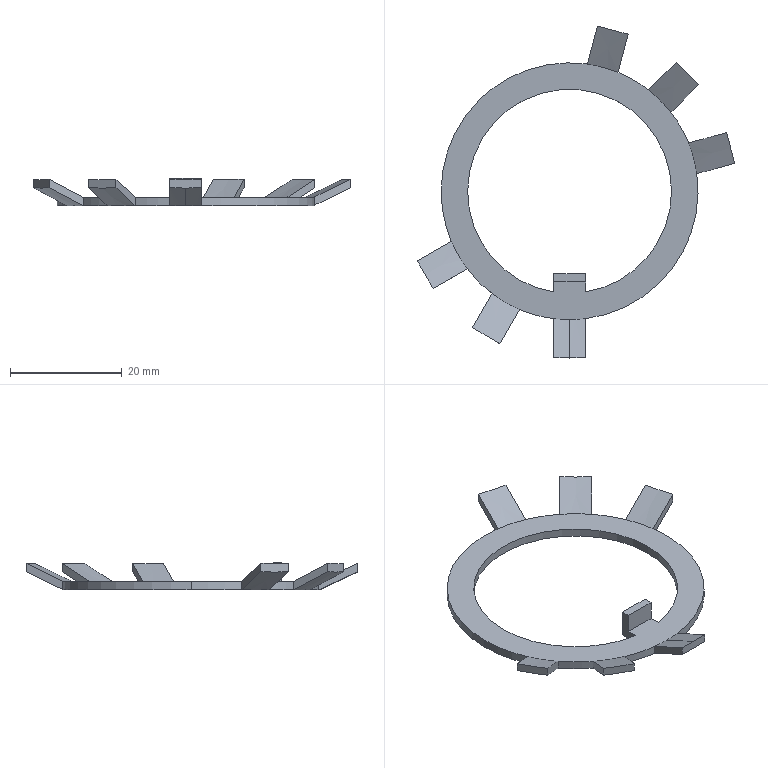Part | SolidWorks | features Boss 1, Cut 1, Revolution 1 | 1 solid | 49 faces | box 56.873 x 59.449 x 5 mm | volume 1338 mm3 | plane 25 | cone 14 | cylinder 10 | commonest cylinder face diameters 46 x7 36.5 x3
STEP:
#1=CARTESIAN_POINT('',(0.,-23.,0.));
#2=VERTEX_POINT('',#1);
#3=CARTESIAN_POINT('',(-2.85,-22.823,0.));
#4=VERTEX_POINT('',#3);
#5=CARTESIAN_POINT('',(0.,0.,0.));
#6=DIRECTION('',(0.,0.,-1.));
#7=DIRECTION('',(0.,1.,0.));
#8=AXIS2_PLACEMENT_3D('',#5,#6,#7);
#9=CIRCLE('',#8,23.);
#10=EDGE_CURVE('',#2,#4,#9,.T.);
#11=ORIENTED_EDGE('',*,*,#10,.F.);
#12=CARTESIAN_POINT('',(0.,-29.864,3.201));
#13=VERTEX_POINT('',#12);
#14=CARTESIAN_POINT('',(0.,-23.,0.));
#15=DIRECTION('',(0.,-0.9063,0.4226));
#16=VECTOR('',#15,1000.);
#17=LINE('',#14,#16);
#18=EDGE_CURVE('',#2,#13,#17,.T.);
#19=ORIENTED_EDGE('',*,*,#18,.T.);
#20=CARTESIAN_POINT('',(-2.85,-29.864,3.264));
#21=VERTEX_POINT('',#20);
#22=CARTESIAN_POINT('',(0.,-29.864,3.201));
#23=CARTESIAN_POINT('',(-0.9489,-29.864,3.201));
#24=CARTESIAN_POINT('',(-1.9,-29.864,3.222));
#25=CARTESIAN_POINT('',(-2.85,-29.864,3.264));
#26=B_SPLINE_CURVE_WITH_KNOTS('',3,(#22,#23,#24,#25),.UNSPECIFIED.,.F.,.F.,(4,4),(0.01086,0.0137),.UNSPECIFIED.);
#27=EDGE_CURVE('',#13,#21,#26,.T.);
#28=ORIENTED_EDGE('',*,*,#27,.T.);
#29=CARTESIAN_POINT('',(-2.85,-29.864,3.264));
#30=CARTESIAN_POINT('',(-2.85,-27.518,2.175));
#31=CARTESIAN_POINT('',(-2.85,-25.171,1.086));
#32=CARTESIAN_POINT('',(-2.85,-22.823,0.));
#33=B_SPLINE_CURVE_WITH_KNOTS('',3,(#29,#30,#31,#32),.UNSPECIFIED.,.F.,.F.,(4,4),(0.01434,0.02211),.UNSPECIFIED.);
#34=EDGE_CURVE('',#21,#4,#33,.T.);
#35=ORIENTED_EDGE('',*,*,#34,.T.);
#36=EDGE_LOOP('',(#11,#19,#28,#35));
#37=FACE_OUTER_BOUND('',#36,.T.);
#38=CARTESIAN_POINT('',(0.,0.,0.));
#39=DIRECTION('',(0.,0.,1.));
#40=DIRECTION('',(0.,-1.,0.));
#41=AXIS2_PLACEMENT_3D('',#38,#39,#40);
#42=CONICAL_SURFACE('',#41,23.,1.134);
#43=ADVANCED_FACE('',(#37),#42,.T.);
#44=CARTESIAN_POINT('',(-21.19,-8.943,1.5));
#45=VERTEX_POINT('',#44);
#46=CARTESIAN_POINT('',(-23.,0.,1.5));
#47=VERTEX_POINT('',#46);
#48=CARTESIAN_POINT('',(0.,0.,1.5));
#49=DIRECTION('',(0.,0.,-1.));
#50=DIRECTION('',(0.,1.,0.));
#51=AXIS2_PLACEMENT_3D('',#48,#49,#50);
#52=CIRCLE('',#51,23.);
#53=EDGE_CURVE('',#45,#47,#52,.T.);
#54=ORIENTED_EDGE('',*,*,#53,.T.);
#55=CARTESIAN_POINT('',(-23.,0.,0.));
#56=VERTEX_POINT('',#55);
#57=CARTESIAN_POINT('',(-23.,0.,4.765));
#58=DIRECTION('',(0.,0.,-1.));
#59=VECTOR('',#58,1000.);
#60=LINE('',#57,#59);
#61=EDGE_CURVE('',#47,#56,#60,.T.);
#62=ORIENTED_EDGE('',*,*,#61,.T.);
#63=CARTESIAN_POINT('',(-21.19,-8.943,0.));
#64=VERTEX_POINT('',#63);
#65=CARTESIAN_POINT('',(0.,0.,0.));
#66=DIRECTION('',(0.,0.,1.));
#67=DIRECTION('',(1.,0.,0.));
#68=AXIS2_PLACEMENT_3D('',#65,#66,#67);
#69=CIRCLE('',#68,23.);
#70=EDGE_CURVE('',#56,#64,#69,.T.);
#71=ORIENTED_EDGE('',*,*,#70,.T.);
#72=CARTESIAN_POINT('',(-21.19,-8.943,4.765));
#73=DIRECTION('',(0.,0.,-1.));
#74=VECTOR('',#73,1000.);
#75=LINE('',#72,#74);
#76=EDGE_CURVE('',#45,#64,#75,.T.);
#77=ORIENTED_EDGE('',*,*,#76,.F.);
#78=EDGE_LOOP('',(#54,#62,#71,#77));
#79=FACE_OUTER_BOUND('',#78,.T.);
#80=CARTESIAN_POINT('',(0.,0.,4.765));
#81=DIRECTION('',(0.,0.,-1.));
#82=DIRECTION('',(-1.,0.,0.));
#83=AXIS2_PLACEMENT_3D('',#80,#81,#82);
#84=CYLINDRICAL_SURFACE('',#83,23.);
#85=ADVANCED_FACE('',(#79),#84,.T.);
#86=CARTESIAN_POINT('',(2.85,-18.026,1.5));
#87=VERTEX_POINT('',#86);
#88=CARTESIAN_POINT('',(18.25,0.,1.5));
#89=VERTEX_POINT('',#88);
#90=CARTESIAN_POINT('',(0.,0.,1.5));
#91=DIRECTION('',(0.,0.,1.));
#92=DIRECTION('',(0.,-1.,0.));
#93=AXIS2_PLACEMENT_3D('',#90,#91,#92);
#94=CIRCLE('',#93,18.25);
#95=EDGE_CURVE('',#87,#89,#94,.T.);
#96=ORIENTED_EDGE('',*,*,#95,.T.);
#97=CARTESIAN_POINT('',(18.25,0.,0.));
#98=VERTEX_POINT('',#97);
#99=CARTESIAN_POINT('',(18.25,0.,4.765));
#100=DIRECTION('',(0.,0.,-1.));
#101=VECTOR('',#100,1000.);
#102=LINE('',#99,#101);
#103=EDGE_CURVE('',#89,#98,#102,.T.);
#104=ORIENTED_EDGE('',*,*,#103,.T.);
#105=CARTESIAN_POINT('',(2.85,-18.026,0.));
#106=VERTEX_POINT('',#105);
#107=CARTESIAN_POINT('',(0.,0.,0.));
#108=DIRECTION('',(0.,0.,1.));
#109=DIRECTION('',(1.,0.,0.));
#110=AXIS2_PLACEMENT_3D('',#107,#108,#109);
#111=CIRCLE('',#110,18.25);
#112=EDGE_CURVE('',#106,#98,#111,.T.);
#113=ORIENTED_EDGE('',*,*,#112,.F.);
#114=CARTESIAN_POINT('',(2.85,-18.026,4.765));
#115=DIRECTION('',(0.,0.,-1.));
#116=VECTOR('',#115,1000.);
#117=LINE('',#114,#116);
#118=EDGE_CURVE('',#87,#106,#117,.T.);
#119=ORIENTED_EDGE('',*,*,#118,.F.);
#120=EDGE_LOOP('',(#96,#104,#113,#119));
#121=FACE_OUTER_BOUND('',#120,.T.);
#122=CARTESIAN_POINT('',(0.,0.,4.765));
#123=DIRECTION('',(0.,0.,-1.));
#124=DIRECTION('',(-1.,0.,0.));
#125=AXIS2_PLACEMENT_3D('',#122,#123,#124);
#126=CYLINDRICAL_SURFACE('',#125,18.25);
#127=ADVANCED_FACE('',(#121),#126,.F.);
#128=ORIENTED_EDGE('',*,*,#103,.F.);
#129=CARTESIAN_POINT('',(-18.25,0.,1.5));
#130=VERTEX_POINT('',#129);
#131=CARTESIAN_POINT('',(0.,0.,1.5));
#132=DIRECTION('',(0.,0.,1.));
#133=DIRECTION('',(0.,-1.,0.));
#134=AXIS2_PLACEMENT_3D('',#131,#132,#133);
#135=CIRCLE('',#134,18.25);
#136=EDGE_CURVE('',#89,#130,#135,.T.);
#137=ORIENTED_EDGE('',*,*,#136,.T.);
#138=CARTESIAN_POINT('',(-18.25,0.,0.));
#139=VERTEX_POINT('',#138);
#140=CARTESIAN_POINT('',(-18.25,0.,4.765));
#141=DIRECTION('',(0.,0.,-1.));
#142=VECTOR('',#141,1000.);
#143=LINE('',#140,#142);
#144=EDGE_CURVE('',#130,#139,#143,.T.);
#145=ORIENTED_EDGE('',*,*,#144,.T.);
#146=CARTESIAN_POINT('',(0.,0.,0.));
#147=DIRECTION('',(0.,0.,1.));
#148=DIRECTION('',(1.,0.,0.));
#149=AXIS2_PLACEMENT_3D('',#146,#147,#148);
#150=CIRCLE('',#149,18.25);
#151=EDGE_CURVE('',#98,#139,#150,.T.);
#152=ORIENTED_EDGE('',*,*,#151,.F.);
#153=EDGE_LOOP('',(#128,#137,#145,#152));
#154=FACE_OUTER_BOUND('',#153,.T.);
#155=CARTESIAN_POINT('',(0.,0.,4.765));
#156=DIRECTION('',(0.,0.,-1.));
#157=DIRECTION('',(-1.,0.,0.));
#158=AXIS2_PLACEMENT_3D('',#155,#156,#157);
#159=CYLINDRICAL_SURFACE('',#158,18.25);
#160=ADVANCED_FACE('',(#154),#159,.F.);
#161=CARTESIAN_POINT('',(2.85,-22.823,1.5));
#162=VERTEX_POINT('',#161);
#163=CARTESIAN_POINT('',(0.,-23.,1.5));
#164=VERTEX_POINT('',#163);
#165=CARTESIAN_POINT('',(0.,0.,1.5));
#166=DIRECTION('',(0.,0.,-1.));
#167=DIRECTION('',(0.,1.,0.));
#168=AXIS2_PLACEMENT_3D('',#165,#166,#167);
#169=CIRCLE('',#168,23.);
#170=EDGE_CURVE('',#162,#164,#169,.T.);
#171=ORIENTED_EDGE('',*,*,#170,.T.);
#172=CARTESIAN_POINT('',(0.,-29.864,4.701));
#173=VERTEX_POINT('',#172);
#174=CARTESIAN_POINT('',(0.,-30.,4.764));
#175=DIRECTION('',(0.,-0.9063,0.4226));
#176=VECTOR('',#175,1000.);
#177=LINE('',#174,#176);
#178=EDGE_CURVE('',#164,#173,#177,.T.);
#179=ORIENTED_EDGE('',*,*,#178,.T.);
#180=CARTESIAN_POINT('',(2.85,-29.864,4.764));
#181=VERTEX_POINT('',#180);
#182=CARTESIAN_POINT('',(0.,-29.864,4.701));
#183=CARTESIAN_POINT('',(0.9514,-29.864,4.701));
#184=CARTESIAN_POINT('',(1.901,-29.864,4.722));
#185=CARTESIAN_POINT('',(2.85,-29.864,4.764));
#186=B_SPLINE_CURVE_WITH_KNOTS('',3,(#182,#183,#184,#185),.UNSPECIFIED.,.F.,.F.,(4,4),(0.01506,0.01791),.UNSPECIFIED.);
#187=EDGE_CURVE('',#173,#181,#186,.T.);
#188=ORIENTED_EDGE('',*,*,#187,.T.);
#189=CARTESIAN_POINT('',(2.85,-29.864,4.764));
#190=CARTESIAN_POINT('',(2.85,-27.518,3.675));
#191=CARTESIAN_POINT('',(2.85,-25.171,2.586));
#192=CARTESIAN_POINT('',(2.85,-22.823,1.5));
#193=B_SPLINE_CURVE_WITH_KNOTS('',3,(#189,#190,#191,#192),.UNSPECIFIED.,.F.,.F.,(4,4),(0.01434,0.02211),.UNSPECIFIED.);
#194=EDGE_CURVE('',#181,#162,#193,.T.);
#195=ORIENTED_EDGE('',*,*,#194,.T.);
#196=EDGE_LOOP('',(#171,#179,#188,#195));
#197=FACE_OUTER_BOUND('',#196,.T.);
#198=CARTESIAN_POINT('',(0.,0.,4.764));
#199=DIRECTION('',(0.,0.,1.));
#200=DIRECTION('',(0.,-1.,0.));
#201=AXIS2_PLACEMENT_3D('',#198,#199,#200);
#202=CONICAL_SURFACE('',#201,30.,1.134);
#203=ADVANCED_FACE('',(#197),#202,.F.);
#204=CARTESIAN_POINT('',(3.154,22.783,1.5));
#205=VERTEX_POINT('',#204);
#206=CARTESIAN_POINT('',(8.66,21.307,1.5));
#207=VERTEX_POINT('',#206);
#208=CARTESIAN_POINT('',(0.,0.,1.5));
#209=DIRECTION('',(0.,0.,-1.));
#210=DIRECTION('',(0.,1.,0.));
#211=AXIS2_PLACEMENT_3D('',#208,#209,#210);
#212=CIRCLE('',#211,23.);
#213=EDGE_CURVE('',#205,#207,#212,.T.);
#214=ORIENTED_EDGE('',*,*,#213,.F.);
#215=CARTESIAN_POINT('',(0.,0.,1.5));
#216=DIRECTION('',(0.,0.,-1.));
#217=DIRECTION('',(0.,1.,0.));
#218=AXIS2_PLACEMENT_3D('',#215,#216,#217);
#219=CIRCLE('',#218,23.);
#220=EDGE_CURVE('',#47,#205,#219,.T.);
#221=ORIENTED_EDGE('',*,*,#220,.F.);
#222=ORIENTED_EDGE('',*,*,#53,.F.);
#223=CARTESIAN_POINT('',(-18.34,-13.88,1.5));
#224=VERTEX_POINT('',#223);
#225=CARTESIAN_POINT('',(0.,0.,1.5));
#226=DIRECTION('',(0.,0.,-1.));
#227=DIRECTION('',(0.,1.,0.));
#228=AXIS2_PLACEMENT_3D('',#225,#226,#227);
#229=CIRCLE('',#228,23.);
#230=EDGE_CURVE('',#224,#45,#229,.T.);
#231=ORIENTED_EDGE('',*,*,#230,.F.);
#232=CARTESIAN_POINT('',(-13.88,-18.34,1.5));
#233=VERTEX_POINT('',#232);
#234=CARTESIAN_POINT('',(0.,0.,1.5));
#235=DIRECTION('',(0.,0.,-1.));
#236=DIRECTION('',(0.,1.,0.));
#237=AXIS2_PLACEMENT_3D('',#234,#235,#236);
#238=CIRCLE('',#237,23.);
#239=EDGE_CURVE('',#233,#224,#238,.T.);
#240=ORIENTED_EDGE('',*,*,#239,.F.);
#241=CARTESIAN_POINT('',(-8.943,-21.19,1.5));
#242=VERTEX_POINT('',#241);
#243=CARTESIAN_POINT('',(0.,0.,1.5));
#244=DIRECTION('',(0.,0.,-1.));
#245=DIRECTION('',(0.,1.,0.));
#246=AXIS2_PLACEMENT_3D('',#243,#244,#245);
#247=CIRCLE('',#246,23.);
#248=EDGE_CURVE('',#242,#233,#247,.T.);
#249=ORIENTED_EDGE('',*,*,#248,.F.);
#250=CARTESIAN_POINT('',(-2.85,-22.823,1.5));
#251=VERTEX_POINT('',#250);
#252=CARTESIAN_POINT('',(0.,0.,1.5));
#253=DIRECTION('',(0.,0.,-1.));
#254=DIRECTION('',(0.,1.,0.));
#255=AXIS2_PLACEMENT_3D('',#252,#253,#254);
#256=CIRCLE('',#255,23.);
#257=EDGE_CURVE('',#251,#242,#256,.T.);
#258=ORIENTED_EDGE('',*,*,#257,.F.);
#259=CARTESIAN_POINT('',(0.,0.,1.5));
#260=DIRECTION('',(0.,0.,-1.));
#261=DIRECTION('',(0.,1.,0.));
#262=AXIS2_PLACEMENT_3D('',#259,#260,#261);
#263=CIRCLE('',#262,23.);
#264=EDGE_CURVE('',#164,#251,#263,.T.);
#265=ORIENTED_EDGE('',*,*,#264,.F.);
#266=ORIENTED_EDGE('',*,*,#170,.F.);
#267=CARTESIAN_POINT('',(22.783,3.154,1.5));
#268=VERTEX_POINT('',#267);
#269=CARTESIAN_POINT('',(0.,0.,1.5));
#270=DIRECTION('',(0.,0.,-1.));
#271=DIRECTION('',(0.,1.,0.));
#272=AXIS2_PLACEMENT_3D('',#269,#270,#271);
#273=CIRCLE('',#272,23.);
#274=EDGE_CURVE('',#268,#162,#273,.T.);
#275=ORIENTED_EDGE('',*,*,#274,.F.);
#276=CARTESIAN_POINT('',(21.307,8.66,1.5));
#277=VERTEX_POINT('',#276);
#278=CARTESIAN_POINT('',(0.,0.,1.5));
#279=DIRECTION('',(0.,0.,-1.));
#280=DIRECTION('',(0.,1.,0.));
#281=AXIS2_PLACEMENT_3D('',#278,#279,#280);
#282=CIRCLE('',#281,23.);
#283=EDGE_CURVE('',#277,#268,#282,.T.);
#284=ORIENTED_EDGE('',*,*,#283,.F.);
#285=CARTESIAN_POINT('',(18.153,14.123,1.5));
#286=VERTEX_POINT('',#285);
#287=CARTESIAN_POINT('',(0.,0.,1.5));
#288=DIRECTION('',(0.,0.,-1.));
#289=DIRECTION('',(0.,1.,0.));
#290=AXIS2_PLACEMENT_3D('',#287,#288,#289);
#291=CIRCLE('',#290,23.);
#292=EDGE_CURVE('',#286,#277,#291,.T.);
#293=ORIENTED_EDGE('',*,*,#292,.F.);
#294=CARTESIAN_POINT('',(14.123,18.153,1.5));
#295=VERTEX_POINT('',#294);
#296=CARTESIAN_POINT('',(0.,0.,1.5));
#297=DIRECTION('',(0.,0.,-1.));
#298=DIRECTION('',(0.,1.,0.));
#299=AXIS2_PLACEMENT_3D('',#296,#297,#298);
#300=CIRCLE('',#299,23.);
#301=EDGE_CURVE('',#295,#286,#300,.T.);
#302=ORIENTED_EDGE('',*,*,#301,.F.);
#303=CARTESIAN_POINT('',(0.,0.,1.5));
#304=DIRECTION('',(0.,0.,-1.));
#305=DIRECTION('',(0.,1.,0.));
#306=AXIS2_PLACEMENT_3D('',#303,#304,#305);
#307=CIRCLE('',#306,23.);
#308=EDGE_CURVE('',#207,#295,#307,.T.);
#309=ORIENTED_EDGE('',*,*,#308,.F.);
#310=EDGE_LOOP('',(#214,#221,#222,#231,#240,#249,#258,#265,#266,#275,#284,#293,#302,#309));
#311=FACE_OUTER_BOUND('',#310,.T.);
#312=CARTESIAN_POINT('',(2.85,-16.25,1.5));
#313=VERTEX_POINT('',#312);
#314=CARTESIAN_POINT('',(2.85,-18.026,1.5));
#315=DIRECTION('',(0.,-1.,0.));
#316=VECTOR('',#315,1000.);
#317=LINE('',#314,#316);
#318=EDGE_CURVE('',#313,#87,#317,.T.);
#319=ORIENTED_EDGE('',*,*,#318,.F.);
#320=CARTESIAN_POINT('',(-2.85,-16.25,1.5));
#321=VERTEX_POINT('',#320);
#322=CARTESIAN_POINT('',(0.,-16.25,1.5));
#323=DIRECTION('',(-1.,0.,0.));
#324=VECTOR('',#323,1000.);
#325=LINE('',#322,#324);
#326=EDGE_CURVE('',#313,#321,#325,.T.);
#327=ORIENTED_EDGE('',*,*,#326,.T.);
#328=CARTESIAN_POINT('',(-2.85,-18.026,1.5));
#329=VERTEX_POINT('',#328);
#330=CARTESIAN_POINT('',(-2.85,-18.026,1.5));
#331=DIRECTION('',(0.,1.,0.));
#332=VECTOR('',#331,1000.);
#333=LINE('',#330,#332);
#334=EDGE_CURVE('',#329,#321,#333,.T.);
#335=ORIENTED_EDGE('',*,*,#334,.F.);
#336=CARTESIAN_POINT('',(0.,0.,1.5));
#337=DIRECTION('',(0.,0.,1.));
#338=DIRECTION('',(0.,-1.,0.));
#339=AXIS2_PLACEMENT_3D('',#336,#337,#338);
#340=CIRCLE('',#339,18.25);
#341=EDGE_CURVE('',#130,#329,#340,.T.);
#342=ORIENTED_EDGE('',*,*,#341,.F.);
#343=ORIENTED_EDGE('',*,*,#136,.F.);
#344=ORIENTED_EDGE('',*,*,#95,.F.);
#345=EDGE_LOOP('',(#319,#327,#335,#342,#343,#344));
#346=FACE_BOUND('',#345,.T.);
#347=CARTESIAN_POINT('',(0.,23.,1.5));
#348=DIRECTION('',(0.,0.,1.));
#349=DIRECTION('',(0.,-1.,0.));
#350=AXIS2_PLACEMENT_3D('',#347,#348,#349);
#351=PLANE('',#350);
#352=ADVANCED_FACE('',(#311,#346),#351,.T.);
#353=ORIENTED_EDGE('',*,*,#178,.F.);
#354=ORIENTED_EDGE('',*,*,#264,.T.);
#355=CARTESIAN_POINT('',(-2.85,-29.864,4.764));
#356=VERTEX_POINT('',#355);
#357=CARTESIAN_POINT('',(-2.85,-22.823,1.5));
#358=CARTESIAN_POINT('',(-2.85,-25.171,2.586));
#359=CARTESIAN_POINT('',(-2.85,-27.518,3.675));
#360=CARTESIAN_POINT('',(-2.85,-29.864,4.764));
#361=B_SPLINE_CURVE_WITH_KNOTS('',3,(#357,#358,#359,#360),.UNSPECIFIED.,.F.,.F.,(4,4),(0.008867,0.01663),.UNSPECIFIED.);
#362=EDGE_CURVE('',#251,#356,#361,.T.);
#363=ORIENTED_EDGE('',*,*,#362,.T.);
#364=CARTESIAN_POINT('',(-2.85,-29.864,4.764));
#365=CARTESIAN_POINT('',(-1.9,-29.864,4.722));
#366=CARTESIAN_POINT('',(-0.9489,-29.864,4.701));
#367=CARTESIAN_POINT('',(0.,-29.864,4.701));
#368=B_SPLINE_CURVE_WITH_KNOTS('',3,(#364,#365,#366,#367),.UNSPECIFIED.,.F.,.F.,(4,4),(0.01222,0.01506),.UNSPECIFIED.);
#369=EDGE_CURVE('',#356,#173,#368,.T.);
#370=ORIENTED_EDGE('',*,*,#369,.T.);
#371=EDGE_LOOP('',(#353,#354,#363,#370));
#372=FACE_OUTER_BOUND('',#371,.T.);
#373=CARTESIAN_POINT('',(0.,0.,4.764));
#374=DIRECTION('',(0.,0.,1.));
#375=DIRECTION('',(0.,-1.,0.));
#376=AXIS2_PLACEMENT_3D('',#373,#374,#375);
#377=CONICAL_SURFACE('',#376,30.,1.134);
#378=ADVANCED_FACE('',(#372),#377,.F.);
#379=CARTESIAN_POINT('',(-17.4,-24.438,4.764));
#380=VERTEX_POINT('',#379);
#381=CARTESIAN_POINT('',(-13.88,-18.34,1.5));
#382=CARTESIAN_POINT('',(-15.054,-20.373,2.586));
#383=CARTESIAN_POINT('',(-16.227,-22.406,3.675));
#384=CARTESIAN_POINT('',(-17.4,-24.438,4.764));
#385=B_SPLINE_CURVE_WITH_KNOTS('',3,(#381,#382,#383,#384),.UNSPECIFIED.,.F.,.F.,(4,4),(0.000000255,0.007762),.UNSPECIFIED.);
#386=EDGE_CURVE('',#233,#380,#385,.T.);
#387=ORIENTED_EDGE('',*,*,#386,.T.);
#388=CARTESIAN_POINT('',(-12.464,-27.288,4.764));
#389=VERTEX_POINT('',#388);
#390=CARTESIAN_POINT('',(-17.4,-24.438,4.764));
#391=CARTESIAN_POINT('',(-15.755,-25.388,4.68));
#392=CARTESIAN_POINT('',(-14.109,-26.338,4.68));
#393=CARTESIAN_POINT('',(-12.464,-27.288,4.764));
#394=B_SPLINE_CURVE_WITH_KNOTS('',3,(#390,#391,#392,#393),.UNSPECIFIED.,.F.,.F.,(4,4),(0.000000231,0.0057),.UNSPECIFIED.);
#395=EDGE_CURVE('',#380,#389,#394,.T.);
#396=ORIENTED_EDGE('',*,*,#395,.T.);
#397=CARTESIAN_POINT('',(-12.464,-27.288,4.764));
#398=CARTESIAN_POINT('',(-11.291,-25.256,3.675));
#399=CARTESIAN_POINT('',(-10.117,-23.223,2.586));
#400=CARTESIAN_POINT('',(-8.943,-21.19,1.5));
#401=B_SPLINE_CURVE_WITH_KNOTS('',3,(#397,#398,#399,#400),.UNSPECIFIED.,.F.,.F.,(4,4),(0.000000255,0.007762),.UNSPECIFIED.);
#402=EDGE_CURVE('',#389,#242,#401,.T.);
#403=ORIENTED_EDGE('',*,*,#402,.T.);
#404=ORIENTED_EDGE('',*,*,#248,.T.);
#405=EDGE_LOOP('',(#387,#396,#403,#404));
#406=FACE_OUTER_BOUND('',#405,.T.);
#407=CARTESIAN_POINT('',(0.,0.,4.764));
#408=DIRECTION('',(0.,0.,1.));
#409=DIRECTION('',(0.,-1.,0.));
#410=AXIS2_PLACEMENT_3D('',#407,#408,#409);
#411=CONICAL_SURFACE('',#410,30.,1.134);
#412=ADVANCED_FACE('',(#406),#411,.F.);
#413=CARTESIAN_POINT('',(-27.288,-12.464,4.764));
#414=VERTEX_POINT('',#413);
#415=CARTESIAN_POINT('',(-21.19,-8.943,1.5));
#416=CARTESIAN_POINT('',(-23.223,-10.117,2.586));
#417=CARTESIAN_POINT('',(-25.256,-11.291,3.675));
#418=CARTESIAN_POINT('',(-27.288,-12.464,4.764));
#419=B_SPLINE_CURVE_WITH_KNOTS('',3,(#415,#416,#417,#418),.UNSPECIFIED.,.F.,.F.,(4,4),(0.000000255,0.007762),.UNSPECIFIED.);
#420=EDGE_CURVE('',#45,#414,#419,.T.);
#421=ORIENTED_EDGE('',*,*,#420,.T.);
#422=CARTESIAN_POINT('',(-24.438,-17.4,4.764));
#423=VERTEX_POINT('',#422);
#424=CARTESIAN_POINT('',(-27.288,-12.464,4.764));
#425=CARTESIAN_POINT('',(-26.338,-14.109,4.68));
#426=CARTESIAN_POINT('',(-25.388,-15.755,4.68));
#427=CARTESIAN_POINT('',(-24.438,-17.4,4.764));
#428=B_SPLINE_CURVE_WITH_KNOTS('',3,(#424,#425,#426,#427),.UNSPECIFIED.,.F.,.F.,(4,4),(0.000000231,0.0057),.UNSPECIFIED.);
#429=EDGE_CURVE('',#414,#423,#428,.T.);
#430=ORIENTED_EDGE('',*,*,#429,.T.);
#431=CARTESIAN_POINT('',(-24.438,-17.4,4.764));
#432=CARTESIAN_POINT('',(-22.406,-16.227,3.675));
#433=CARTESIAN_POINT('',(-20.373,-15.054,2.586));
#434=CARTESIAN_POINT('',(-18.34,-13.88,1.5));
#435=B_SPLINE_CURVE_WITH_KNOTS('',3,(#431,#432,#433,#434),.UNSPECIFIED.,.F.,.F.,(4,4),(0.000000255,0.007762),.UNSPECIFIED.);
#436=EDGE_CURVE('',#423,#224,#435,.T.);
#437=ORIENTED_EDGE('',*,*,#436,.T.);
#438=ORIENTED_EDGE('',*,*,#230,.T.);
#439=EDGE_LOOP('',(#421,#430,#437,#438));
#440=FACE_OUTER_BOUND('',#439,.T.);
#441=CARTESIAN_POINT('',(0.,0.,4.764));
#442=DIRECTION('',(0.,0.,1.));
#443=DIRECTION('',(0.,-1.,0.));
#444=AXIS2_PLACEMENT_3D('',#441,#442,#443);
#445=CONICAL_SURFACE('',#444,30.,1.134);
#446=ADVANCED_FACE('',(#440),#445,.F.);
#447=CARTESIAN_POINT('',(10.482,28.109,4.764));
#448=VERTEX_POINT('',#447);
#449=CARTESIAN_POINT('',(8.66,21.307,1.5));
#450=CARTESIAN_POINT('',(9.268,23.575,2.586));
#451=CARTESIAN_POINT('',(9.875,25.842,3.675));
#452=CARTESIAN_POINT('',(10.482,28.109,4.764));
#453=B_SPLINE_CURVE_WITH_KNOTS('',3,(#449,#450,#451,#452),.UNSPECIFIED.,.F.,.F.,(4,4),(0.000000228,0.007762),.UNSPECIFIED.);
#454=EDGE_CURVE('',#207,#448,#453,.T.);
#455=ORIENTED_EDGE('',*,*,#454,.T.);
#456=CARTESIAN_POINT('',(4.977,29.584,4.764));
#457=VERTEX_POINT('',#456);
#458=CARTESIAN_POINT('',(10.482,28.109,4.764));
#459=CARTESIAN_POINT('',(8.647,28.601,4.68));
#460=CARTESIAN_POINT('',(6.812,29.093,4.68));
#461=CARTESIAN_POINT('',(4.977,29.584,4.764));
#462=B_SPLINE_CURVE_WITH_KNOTS('',3,(#458,#459,#460,#461),.UNSPECIFIED.,.F.,.F.,(4,4),(0.000000207,0.0057),.UNSPECIFIED.);
#463=EDGE_CURVE('',#448,#457,#462,.T.);
#464=ORIENTED_EDGE('',*,*,#463,.T.);
#465=CARTESIAN_POINT('',(4.977,29.584,4.764));
#466=CARTESIAN_POINT('',(4.369,27.318,3.675));
#467=CARTESIAN_POINT('',(3.762,25.051,2.586));
#468=CARTESIAN_POINT('',(3.154,22.783,1.5));
#469=B_SPLINE_CURVE_WITH_KNOTS('',3,(#465,#466,#467,#468),.UNSPECIFIED.,.F.,.F.,(4,4),(0.000000228,0.007762),.UNSPECIFIED.);
#470=EDGE_CURVE('',#457,#205,#469,.T.);
#471=ORIENTED_EDGE('',*,*,#470,.T.);
#472=ORIENTED_EDGE('',*,*,#213,.T.);
#473=EDGE_LOOP('',(#455,#464,#471,#472));
#474=FACE_OUTER_BOUND('',#473,.T.);
#475=CARTESIAN_POINT('',(0.,0.,4.764));
#476=DIRECTION('',(0.,0.,1.));
#477=DIRECTION('',(0.,-1.,0.));
#478=AXIS2_PLACEMENT_3D('',#475,#476,#477);
#479=CONICAL_SURFACE('',#478,30.,1.134);
#480=ADVANCED_FACE('',(#474),#479,.F.);
#481=CARTESIAN_POINT('',(23.133,19.102,4.764));
#482=VERTEX_POINT('',#481);
#483=CARTESIAN_POINT('',(18.153,14.123,1.5));
#484=CARTESIAN_POINT('',(19.814,15.783,2.586));
#485=CARTESIAN_POINT('',(21.473,17.443,3.675));
#486=CARTESIAN_POINT('',(23.133,19.102,4.764));
#487=B_SPLINE_CURVE_WITH_KNOTS('',3,(#483,#484,#485,#486),.UNSPECIFIED.,.F.,.F.,(4,4),(0.000000312,0.007762),.UNSPECIFIED.);
#488=EDGE_CURVE('',#286,#482,#487,.T.);
#489=ORIENTED_EDGE('',*,*,#488,.T.);
#490=CARTESIAN_POINT('',(19.102,23.133,4.764));
#491=VERTEX_POINT('',#490);
#492=CARTESIAN_POINT('',(23.133,19.102,4.764));
#493=CARTESIAN_POINT('',(21.789,20.446,4.68));
#494=CARTESIAN_POINT('',(20.446,21.789,4.68));
#495=CARTESIAN_POINT('',(19.102,23.133,4.764));
#496=B_SPLINE_CURVE_WITH_KNOTS('',3,(#492,#493,#494,#495),.UNSPECIFIED.,.F.,.F.,(4,4),(0.000000283,0.0057),.UNSPECIFIED.);
#497=EDGE_CURVE('',#482,#491,#496,.T.);
#498=ORIENTED_EDGE('',*,*,#497,.T.);
#499=CARTESIAN_POINT('',(19.102,23.133,4.764));
#500=CARTESIAN_POINT('',(17.443,21.473,3.675));
#501=CARTESIAN_POINT('',(15.783,19.814,2.586));
#502=CARTESIAN_POINT('',(14.123,18.153,1.5));
#503=B_SPLINE_CURVE_WITH_KNOTS('',3,(#499,#500,#501,#502),.UNSPECIFIED.,.F.,.F.,(4,4),(0.000000312,0.007762),.UNSPECIFIED.);
#504=EDGE_CURVE('',#491,#295,#503,.T.);
#505=ORIENTED_EDGE('',*,*,#504,.T.);
#506=ORIENTED_EDGE('',*,*,#301,.T.);
#507=EDGE_LOOP('',(#489,#498,#505,#506));
#508=FACE_OUTER_BOUND('',#507,.T.);
#509=CARTESIAN_POINT('',(0.,0.,4.764));
#510=DIRECTION('',(0.,0.,1.));
#511=DIRECTION('',(0.,-1.,0.));
#512=AXIS2_PLACEMENT_3D('',#509,#510,#511);
#513=CONICAL_SURFACE('',#512,30.,1.134);
#514=ADVANCED_FACE('',(#508),#513,.F.);
#515=CARTESIAN_POINT('',(29.584,4.977,4.764));
#516=VERTEX_POINT('',#515);
#517=CARTESIAN_POINT('',(22.783,3.154,1.5));
#518=CARTESIAN_POINT('',(25.051,3.762,2.586));
#519=CARTESIAN_POINT('',(27.318,4.369,3.675));
#520=CARTESIAN_POINT('',(29.584,4.977,4.764));
#521=B_SPLINE_CURVE_WITH_KNOTS('',3,(#517,#518,#519,#520),.UNSPECIFIED.,.F.,.F.,(4,4),(0.000000228,0.007762),.UNSPECIFIED.);
#522=EDGE_CURVE('',#268,#516,#521,.T.);
#523=ORIENTED_EDGE('',*,*,#522,.T.);
#524=CARTESIAN_POINT('',(28.109,10.482,4.764));
#525=VERTEX_POINT('',#524);
#526=CARTESIAN_POINT('',(29.584,4.977,4.764));
#527=CARTESIAN_POINT('',(29.093,6.812,4.68));
#528=CARTESIAN_POINT('',(28.601,8.647,4.68));
#529=CARTESIAN_POINT('',(28.109,10.482,4.764));
#530=B_SPLINE_CURVE_WITH_KNOTS('',3,(#526,#527,#528,#529),.UNSPECIFIED.,.F.,.F.,(4,4),(0.000000207,0.0057),.UNSPECIFIED.);
#531=EDGE_CURVE('',#516,#525,#530,.T.);
#532=ORIENTED_EDGE('',*,*,#531,.T.);
#533=CARTESIAN_POINT('',(28.109,10.482,4.764));
#534=CARTESIAN_POINT('',(25.842,9.875,3.675));
#535=CARTESIAN_POINT('',(23.575,9.268,2.586));
#536=CARTESIAN_POINT('',(21.307,8.66,1.5));
#537=B_SPLINE_CURVE_WITH_KNOTS('',3,(#533,#534,#535,#536),.UNSPECIFIED.,.F.,.F.,(4,4),(0.000000228,0.007762),.UNSPECIFIED.);
#538=EDGE_CURVE('',#525,#277,#537,.T.);
#539=ORIENTED_EDGE('',*,*,#538,.T.);
#540=ORIENTED_EDGE('',*,*,#283,.T.);
#541=EDGE_LOOP('',(#523,#532,#539,#540));
#542=FACE_OUTER_BOUND('',#541,.T.);
#543=CARTESIAN_POINT('',(0.,0.,4.764));
#544=DIRECTION('',(0.,0.,1.));
#545=DIRECTION('',(0.,-1.,0.));
#546=AXIS2_PLACEMENT_3D('',#543,#544,#545);
#547=CONICAL_SURFACE('',#546,30.,1.134);
#548=ADVANCED_FACE('',(#542),#547,.F.);
#549=CARTESIAN_POINT('',(2.85,-14.75,5.));
#550=VERTEX_POINT('',#549);
#551=CARTESIAN_POINT('',(2.85,-14.75,0.));
#552=VERTEX_POINT('',#551);
#553=CARTESIAN_POINT('',(2.85,-14.75,4.765));
#554=DIRECTION('',(0.,0.,-1.));
#555=VECTOR('',#554,1000.);
#556=LINE('',#553,#555);
#557=EDGE_CURVE('',#550,#552,#556,.T.);
#558=ORIENTED_EDGE('',*,*,#557,.F.);
#559=CARTESIAN_POINT('',(2.85,-16.25,5.));
#560=VERTEX_POINT('',#559);
#561=CARTESIAN_POINT('',(2.85,-14.75,5.));
#562=DIRECTION('',(0.,1.,0.));
#563=VECTOR('',#562,1000.);
#564=LINE('',#561,#563);
#565=EDGE_CURVE('',#560,#550,#564,.T.);
#566=ORIENTED_EDGE('',*,*,#565,.F.);
#567=CARTESIAN_POINT('',(2.85,-16.25,5.));
#568=DIRECTION('',(0.,0.,-1.));
#569=VECTOR('',#568,1000.);
#570=LINE('',#567,#569);
#571=EDGE_CURVE('',#560,#313,#570,.T.);
#572=ORIENTED_EDGE('',*,*,#571,.T.);
#573=ORIENTED_EDGE('',*,*,#318,.T.);
#574=ORIENTED_EDGE('',*,*,#118,.T.);
#575=CARTESIAN_POINT('',(2.85,-18.026,0.));
#576=DIRECTION('',(0.,-1.,0.));
#577=VECTOR('',#576,1000.);
#578=LINE('',#575,#577);
#579=EDGE_CURVE('',#552,#106,#578,.T.);
#580=ORIENTED_EDGE('',*,*,#579,.F.);
#581=EDGE_LOOP('',(#558,#566,#572,#573,#574,#580));
#582=FACE_OUTER_BOUND('',#581,.T.);
#583=CARTESIAN_POINT('',(2.85,-18.026,4.765));
#584=DIRECTION('',(1.,0.,0.));
#585=DIRECTION('',(0.,1.,0.));
#586=AXIS2_PLACEMENT_3D('',#583,#584,#585);
#587=PLANE('',#586);
#588=ADVANCED_FACE('',(#582),#587,.T.);
#589=CARTESIAN_POINT('',(-2.85,-14.75,5.));
#590=VERTEX_POINT('',#589);
#591=CARTESIAN_POINT('',(-2.85,-14.75,0.));
#592=VERTEX_POINT('',#591);
#593=CARTESIAN_POINT('',(-2.85,-14.75,4.765));
#594=DIRECTION('',(0.,0.,-1.));
#595=VECTOR('',#594,1000.);
#596=LINE('',#593,#595);
#597=EDGE_CURVE('',#590,#592,#596,.T.);
#598=ORIENTED_EDGE('',*,*,#597,.F.);
#599=CARTESIAN_POINT('',(-2.85,-14.75,5.));
#600=DIRECTION('',(-1.,0.,0.));
#601=VECTOR('',#600,1000.);
#602=LINE('',#599,#601);
#603=EDGE_CURVE('',#550,#590,#602,.T.);
#604=ORIENTED_EDGE('',*,*,#603,.F.);
#605=ORIENTED_EDGE('',*,*,#557,.T.);
#606=CARTESIAN_POINT('',(2.85,-14.75,0.));
#607=DIRECTION('',(1.,0.,0.));
#608=VECTOR('',#607,1000.);
#609=LINE('',#606,#608);
#610=EDGE_CURVE('',#592,#552,#609,.T.);
#611=ORIENTED_EDGE('',*,*,#610,.F.);
#612=EDGE_LOOP('',(#598,#604,#605,#611));
#613=FACE_OUTER_BOUND('',#612,.T.);
#614=CARTESIAN_POINT('',(2.85,-14.75,4.765));
#615=DIRECTION('',(0.,1.,0.));
#616=DIRECTION('',(0.,0.,1.));
#617=AXIS2_PLACEMENT_3D('',#614,#615,#616);
#618=PLANE('',#617);
#619=ADVANCED_FACE('',(#613),#618,.T.);
#620=ORIENTED_EDGE('',*,*,#597,.T.);
#621=CARTESIAN_POINT('',(-2.85,-18.026,0.));
#622=VERTEX_POINT('',#621);
#623=CARTESIAN_POINT('',(-2.85,-18.026,0.));
#624=DIRECTION('',(0.,1.,0.));
#625=VECTOR('',#624,1000.);
#626=LINE('',#623,#625);
#627=EDGE_CURVE('',#622,#592,#626,.T.);
#628=ORIENTED_EDGE('',*,*,#627,.F.);
#629=CARTESIAN_POINT('',(-2.85,-18.026,4.765));
#630=DIRECTION('',(0.,0.,-1.));
#631=VECTOR('',#630,1000.);
#632=LINE('',#629,#631);
#633=EDGE_CURVE('',#329,#622,#632,.T.);
#634=ORIENTED_EDGE('',*,*,#633,.F.);
#635=ORIENTED_EDGE('',*,*,#334,.T.);
#636=CARTESIAN_POINT('',(-2.85,-16.25,5.));
#637=VERTEX_POINT('',#636);
#638=CARTESIAN_POINT('',(-2.85,-16.25,5.));
#639=DIRECTION('',(0.,0.,-1.));
#640=VECTOR('',#639,1000.);
#641=LINE('',#638,#640);
#642=EDGE_CURVE('',#637,#321,#641,.T.);
#643=ORIENTED_EDGE('',*,*,#642,.F.);
#644=CARTESIAN_POINT('',(-2.85,-14.75,5.));
#645=DIRECTION('',(0.,-1.,0.));
#646=VECTOR('',#645,1000.);
#647=LINE('',#644,#646);
#648=EDGE_CURVE('',#590,#637,#647,.T.);
#649=ORIENTED_EDGE('',*,*,#648,.F.);
#650=EDGE_LOOP('',(#620,#628,#634,#635,#643,#649));
#651=FACE_OUTER_BOUND('',#650,.T.);
#652=CARTESIAN_POINT('',(-2.85,-18.026,4.765));
#653=DIRECTION('',(-1.,0.,0.));
#654=DIRECTION('',(0.,-1.,0.));
#655=AXIS2_PLACEMENT_3D('',#652,#653,#654);
#656=PLANE('',#655);
#657=ADVANCED_FACE('',(#651),#656,.T.);
#658=ORIENTED_EDGE('',*,*,#144,.F.);
#659=ORIENTED_EDGE('',*,*,#341,.T.);
#660=ORIENTED_EDGE('',*,*,#633,.T.);
#661=CARTESIAN_POINT('',(0.,0.,0.));
#662=DIRECTION('',(0.,0.,1.));
#663=DIRECTION('',(1.,0.,0.));
#664=AXIS2_PLACEMENT_3D('',#661,#662,#663);
#665=CIRCLE('',#664,18.25);
#666=EDGE_CURVE('',#139,#622,#665,.T.);
#667=ORIENTED_EDGE('',*,*,#666,.F.);
#668=EDGE_LOOP('',(#658,#659,#660,#667));
#669=FACE_OUTER_BOUND('',#668,.T.);
#670=CARTESIAN_POINT('',(0.,0.,4.765));
#671=DIRECTION('',(0.,0.,-1.));
#672=DIRECTION('',(-1.,0.,0.));
#673=AXIS2_PLACEMENT_3D('',#670,#671,#672);
#674=CYLINDRICAL_SURFACE('',#673,18.25);
#675=ADVANCED_FACE('',(#669),#674,.F.);
#676=CARTESIAN_POINT('',(2.85,-22.823,0.));
#677=VERTEX_POINT('',#676);
#678=CARTESIAN_POINT('',(2.85,-29.864,3.264));
#679=VERTEX_POINT('',#678);
#680=CARTESIAN_POINT('',(2.85,-22.823,0.));
#681=CARTESIAN_POINT('',(2.85,-25.171,1.086));
#682=CARTESIAN_POINT('',(2.85,-27.518,2.175));
#683=CARTESIAN_POINT('',(2.85,-29.864,3.264));
#684=B_SPLINE_CURVE_WITH_KNOTS('',3,(#680,#681,#682,#683),.UNSPECIFIED.,.F.,.F.,(4,4),(0.008867,0.01663),.UNSPECIFIED.);
#685=EDGE_CURVE('',#677,#679,#684,.T.);
#686=ORIENTED_EDGE('',*,*,#685,.F.);
#687=CARTESIAN_POINT('',(2.85,-22.823,4.765));
#688=DIRECTION('',(0.,0.,-1.));
#689=VECTOR('',#688,1000.);
#690=LINE('',#687,#689);
#691=EDGE_CURVE('',#162,#677,#690,.T.);
#692=ORIENTED_EDGE('',*,*,#691,.F.);
#693=ORIENTED_EDGE('',*,*,#194,.F.);
#694=CARTESIAN_POINT('',(2.85,-29.864,4.765));
#695=DIRECTION('',(0.,0.,-1.));
#696=VECTOR('',#695,1000.);
#697=LINE('',#694,#696);
#698=EDGE_CURVE('',#181,#679,#697,.T.);
#699=ORIENTED_EDGE('',*,*,#698,.T.);
#700=EDGE_LOOP('',(#686,#692,#693,#699));
#701=FACE_OUTER_BOUND('',#700,.T.);
#702=CARTESIAN_POINT('',(2.85,-22.823,4.765));
#703=DIRECTION('',(-1.,0.,0.));
#704=DIRECTION('',(0.,-1.,0.));
#705=AXIS2_PLACEMENT_3D('',#702,#703,#704);
#706=PLANE('',#705);
#707=ADVANCED_FACE('',(#701),#706,.F.);
#708=ORIENTED_EDGE('',*,*,#274,.T.);
#709=ORIENTED_EDGE('',*,*,#691,.T.);
#710=CARTESIAN_POINT('',(22.783,3.154,0.));
#711=VERTEX_POINT('',#710);
#712=CARTESIAN_POINT('',(0.,0.,0.));
#713=DIRECTION('',(0.,0.,1.));
#714=DIRECTION('',(1.,0.,0.));
#715=AXIS2_PLACEMENT_3D('',#712,#713,#714);
#716=CIRCLE('',#715,23.);
#717=EDGE_CURVE('',#677,#711,#716,.T.);
#718=ORIENTED_EDGE('',*,*,#717,.T.);
#719=CARTESIAN_POINT('',(22.783,3.154,4.765));
#720=DIRECTION('',(0.,0.,-1.));
#721=VECTOR('',#720,1000.);
#722=LINE('',#719,#721);
#723=EDGE_CURVE('',#268,#711,#722,.T.);
#724=ORIENTED_EDGE('',*,*,#723,.F.);
#725=EDGE_LOOP('',(#708,#709,#718,#724));
#726=FACE_OUTER_BOUND('',#725,.T.);
#727=CARTESIAN_POINT('',(0.,0.,4.765));
#728=DIRECTION('',(0.,0.,-1.));
#729=DIRECTION('',(-1.,0.,0.));
#730=AXIS2_PLACEMENT_3D('',#727,#728,#729);
#731=CYLINDRICAL_SURFACE('',#730,23.);
#732=ADVANCED_FACE('',(#726),#731,.T.);
#733=CARTESIAN_POINT('',(29.584,4.977,3.264));
#734=VERTEX_POINT('',#733);
#735=CARTESIAN_POINT('',(29.584,4.977,3.264));
#736=CARTESIAN_POINT('',(27.318,4.369,2.175));
#737=CARTESIAN_POINT('',(25.051,3.762,1.086));
#738=CARTESIAN_POINT('',(22.783,3.154,0.));
#739=B_SPLINE_CURVE_WITH_KNOTS('',3,(#735,#736,#737,#738),.UNSPECIFIED.,.F.,.F.,(4,4),(0.000000228,0.007762),.UNSPECIFIED.);
#740=EDGE_CURVE('',#734,#711,#739,.T.);
#741=ORIENTED_EDGE('',*,*,#740,.F.);
#742=CARTESIAN_POINT('',(29.584,4.977,4.765));
#743=DIRECTION('',(0.,0.,-1.));
#744=VECTOR('',#743,1000.);
#745=LINE('',#742,#744);
#746=EDGE_CURVE('',#516,#734,#745,.T.);
#747=ORIENTED_EDGE('',*,*,#746,.F.);
#748=ORIENTED_EDGE('',*,*,#522,.F.);
#749=ORIENTED_EDGE('',*,*,#723,.T.);
#750=EDGE_LOOP('',(#741,#747,#748,#749));
#751=FACE_OUTER_BOUND('',#750,.T.);
#752=CARTESIAN_POINT('',(22.783,3.154,4.765));
#753=DIRECTION('',(-0.2588,0.9659,0.));
#754=DIRECTION('',(-0.9659,-0.2588,0.));
#755=AXIS2_PLACEMENT_3D('',#752,#753,#754);
#756=PLANE('',#755);
#757=ADVANCED_FACE('',(#751),#756,.F.);
#758=CARTESIAN_POINT('',(28.109,10.482,3.264));
#759=VERTEX_POINT('',#758);
#760=CARTESIAN_POINT('',(28.109,10.482,3.264));
#761=CARTESIAN_POINT('',(28.601,8.647,3.18));
#762=CARTESIAN_POINT('',(29.093,6.812,3.18));
#763=CARTESIAN_POINT('',(29.584,4.977,3.264));
#764=B_SPLINE_CURVE_WITH_KNOTS('',3,(#760,#761,#762,#763),.UNSPECIFIED.,.F.,.F.,(4,4),(0.000000207,0.0057),.UNSPECIFIED.);
#765=EDGE_CURVE('',#759,#734,#764,.T.);
#766=ORIENTED_EDGE('',*,*,#765,.F.);
#767=CARTESIAN_POINT('',(28.109,10.482,4.765));
#768=DIRECTION('',(0.,0.,-1.));
#769=VECTOR('',#768,1000.);
#770=LINE('',#767,#769);
#771=EDGE_CURVE('',#525,#759,#770,.T.);
#772=ORIENTED_EDGE('',*,*,#771,.F.);
#773=ORIENTED_EDGE('',*,*,#531,.F.);
#774=ORIENTED_EDGE('',*,*,#746,.T.);
#775=EDGE_LOOP('',(#766,#772,#773,#774));
#776=FACE_OUTER_BOUND('',#775,.T.);
#777=CARTESIAN_POINT('',(28.109,10.482,4.765));
#778=DIRECTION('',(-0.9659,-0.2588,0.));
#779=DIRECTION('',(0.2588,-0.9659,0.));
#780=AXIS2_PLACEMENT_3D('',#777,#778,#779);
#781=PLANE('',#780);
#782=ADVANCED_FACE('',(#776),#781,.F.);
#783=CARTESIAN_POINT('',(21.307,8.66,0.));
#784=VERTEX_POINT('',#783);
#785=CARTESIAN_POINT('',(21.307,8.66,0.));
#786=CARTESIAN_POINT('',(23.575,9.268,1.086));
#787=CARTESIAN_POINT('',(25.842,9.875,2.175));
#788=CARTESIAN_POINT('',(28.109,10.482,3.264));
#789=B_SPLINE_CURVE_WITH_KNOTS('',3,(#785,#786,#787,#788),.UNSPECIFIED.,.F.,.F.,(4,4),(0.000000228,0.007762),.UNSPECIFIED.);
#790=EDGE_CURVE('',#784,#759,#789,.T.);
#791=ORIENTED_EDGE('',*,*,#790,.F.);
#792=CARTESIAN_POINT('',(21.307,8.66,4.765));
#793=DIRECTION('',(0.,0.,-1.));
#794=VECTOR('',#793,1000.);
#795=LINE('',#792,#794);
#796=EDGE_CURVE('',#277,#784,#795,.T.);
#797=ORIENTED_EDGE('',*,*,#796,.F.);
#798=ORIENTED_EDGE('',*,*,#538,.F.);
#799=ORIENTED_EDGE('',*,*,#771,.T.);
#800=EDGE_LOOP('',(#791,#797,#798,#799));
#801=FACE_OUTER_BOUND('',#800,.T.);
#802=CARTESIAN_POINT('',(21.307,8.66,4.765));
#803=DIRECTION('',(0.2588,-0.9659,0.));
#804=DIRECTION('',(0.9659,0.2588,0.));
#805=AXIS2_PLACEMENT_3D('',#802,#803,#804);
#806=PLANE('',#805);
#807=ADVANCED_FACE('',(#801),#806,.F.);
#808=ORIENTED_EDGE('',*,*,#292,.T.);
#809=ORIENTED_EDGE('',*,*,#796,.T.);
#810=CARTESIAN_POINT('',(18.153,14.123,0.));
#811=VERTEX_POINT('',#810);
#812=CARTESIAN_POINT('',(0.,0.,0.));
#813=DIRECTION('',(0.,0.,1.));
#814=DIRECTION('',(1.,0.,0.));
#815=AXIS2_PLACEMENT_3D('',#812,#813,#814);
#816=CIRCLE('',#815,23.);
#817=EDGE_CURVE('',#784,#811,#816,.T.);
#818=ORIENTED_EDGE('',*,*,#817,.T.);
#819=CARTESIAN_POINT('',(18.153,14.123,4.765));
#820=DIRECTION('',(0.,0.,-1.));
#821=VECTOR('',#820,1000.);
#822=LINE('',#819,#821);
#823=EDGE_CURVE('',#286,#811,#822,.T.);
#824=ORIENTED_EDGE('',*,*,#823,.F.);
#825=EDGE_LOOP('',(#808,#809,#818,#824));
#826=FACE_OUTER_BOUND('',#825,.T.);
#827=CARTESIAN_POINT('',(0.,0.,4.765));
#828=DIRECTION('',(0.,0.,-1.));
#829=DIRECTION('',(-1.,0.,0.));
#830=AXIS2_PLACEMENT_3D('',#827,#828,#829);
#831=CYLINDRICAL_SURFACE('',#830,23.);
#832=ADVANCED_FACE('',(#826),#831,.T.);
#833=CARTESIAN_POINT('',(23.133,19.102,3.264));
#834=VERTEX_POINT('',#833);
#835=CARTESIAN_POINT('',(23.133,19.102,3.264));
#836=CARTESIAN_POINT('',(21.473,17.443,2.175));
#837=CARTESIAN_POINT('',(19.814,15.783,1.086));
#838=CARTESIAN_POINT('',(18.153,14.123,0.));
#839=B_SPLINE_CURVE_WITH_KNOTS('',3,(#835,#836,#837,#838),.UNSPECIFIED.,.F.,.F.,(4,4),(0.000000312,0.007762),.UNSPECIFIED.);
#840=EDGE_CURVE('',#834,#811,#839,.T.);
#841=ORIENTED_EDGE('',*,*,#840,.F.);
#842=CARTESIAN_POINT('',(23.133,19.102,4.765));
#843=DIRECTION('',(0.,0.,-1.));
#844=VECTOR('',#843,1000.);
#845=LINE('',#842,#844);
#846=EDGE_CURVE('',#482,#834,#845,.T.);
#847=ORIENTED_EDGE('',*,*,#846,.F.);
#848=ORIENTED_EDGE('',*,*,#488,.F.);
#849=ORIENTED_EDGE('',*,*,#823,.T.);
#850=EDGE_LOOP('',(#841,#847,#848,#849));
#851=FACE_OUTER_BOUND('',#850,.T.);
#852=CARTESIAN_POINT('',(18.153,14.123,4.765));
#853=DIRECTION('',(-0.7071,0.7071,0.));
#854=DIRECTION('',(-0.7071,-0.7071,0.));
#855=AXIS2_PLACEMENT_3D('',#852,#853,#854);
#856=PLANE('',#855);
#857=ADVANCED_FACE('',(#851),#856,.F.);
#858=CARTESIAN_POINT('',(19.102,23.133,3.264));
#859=VERTEX_POINT('',#858);
#860=CARTESIAN_POINT('',(19.102,23.133,3.264));
#861=CARTESIAN_POINT('',(20.446,21.789,3.18));
#862=CARTESIAN_POINT('',(21.789,20.446,3.18));
#863=CARTESIAN_POINT('',(23.133,19.102,3.264));
#864=B_SPLINE_CURVE_WITH_KNOTS('',3,(#860,#861,#862,#863),.UNSPECIFIED.,.F.,.F.,(4,4),(0.000000283,0.0057),.UNSPECIFIED.);
#865=EDGE_CURVE('',#859,#834,#864,.T.);
#866=ORIENTED_EDGE('',*,*,#865,.F.);
#867=CARTESIAN_POINT('',(19.102,23.133,4.765));
#868=DIRECTION('',(0.,0.,-1.));
#869=VECTOR('',#868,1000.);
#870=LINE('',#867,#869);
#871=EDGE_CURVE('',#491,#859,#870,.T.);
#872=ORIENTED_EDGE('',*,*,#871,.F.);
#873=ORIENTED_EDGE('',*,*,#497,.F.);
#874=ORIENTED_EDGE('',*,*,#846,.T.);
#875=EDGE_LOOP('',(#866,#872,#873,#874));
#876=FACE_OUTER_BOUND('',#875,.T.);
#877=CARTESIAN_POINT('',(19.102,23.133,4.765));
#878=DIRECTION('',(-0.7071,-0.7071,0.));
#879=DIRECTION('',(0.7071,-0.7071,0.));
#880=AXIS2_PLACEMENT_3D('',#877,#878,#879);
#881=PLANE('',#880);
#882=ADVANCED_FACE('',(#876),#881,.F.);
#883=CARTESIAN_POINT('',(14.123,18.153,0.));
#884=VERTEX_POINT('',#883);
#885=CARTESIAN_POINT('',(14.123,18.153,0.));
#886=CARTESIAN_POINT('',(15.783,19.814,1.086));
#887=CARTESIAN_POINT('',(17.443,21.473,2.175));
#888=CARTESIAN_POINT('',(19.102,23.133,3.264));
#889=B_SPLINE_CURVE_WITH_KNOTS('',3,(#885,#886,#887,#888),.UNSPECIFIED.,.F.,.F.,(4,4),(0.000000312,0.007762),.UNSPECIFIED.);
#890=EDGE_CURVE('',#884,#859,#889,.T.);
#891=ORIENTED_EDGE('',*,*,#890,.F.);
#892=CARTESIAN_POINT('',(14.123,18.153,4.765));
#893=DIRECTION('',(0.,0.,-1.));
#894=VECTOR('',#893,1000.);
#895=LINE('',#892,#894);
#896=EDGE_CURVE('',#295,#884,#895,.T.);
#897=ORIENTED_EDGE('',*,*,#896,.F.);
#898=ORIENTED_EDGE('',*,*,#504,.F.);
#899=ORIENTED_EDGE('',*,*,#871,.T.);
#900=EDGE_LOOP('',(#891,#897,#898,#899));
#901=FACE_OUTER_BOUND('',#900,.T.);
#902=CARTESIAN_POINT('',(14.123,18.153,4.765));
#903=DIRECTION('',(0.7071,-0.7071,0.));
#904=DIRECTION('',(0.7071,0.7071,0.));
#905=AXIS2_PLACEMENT_3D('',#902,#903,#904);
#906=PLANE('',#905);
#907=ADVANCED_FACE('',(#901),#906,.F.);
#908=ORIENTED_EDGE('',*,*,#308,.T.);
#909=ORIENTED_EDGE('',*,*,#896,.T.);
#910=CARTESIAN_POINT('',(8.66,21.307,0.));
#911=VERTEX_POINT('',#910);
#912=CARTESIAN_POINT('',(0.,0.,0.));
#913=DIRECTION('',(0.,0.,1.));
#914=DIRECTION('',(1.,0.,0.));
#915=AXIS2_PLACEMENT_3D('',#912,#913,#914);
#916=CIRCLE('',#915,23.);
#917=EDGE_CURVE('',#884,#911,#916,.T.);
#918=ORIENTED_EDGE('',*,*,#917,.T.);
#919=CARTESIAN_POINT('',(8.66,21.307,4.765));
#920=DIRECTION('',(0.,0.,-1.));
#921=VECTOR('',#920,1000.);
#922=LINE('',#919,#921);
#923=EDGE_CURVE('',#207,#911,#922,.T.);
#924=ORIENTED_EDGE('',*,*,#923,.F.);
#925=EDGE_LOOP('',(#908,#909,#918,#924));
#926=FACE_OUTER_BOUND('',#925,.T.);
#927=CARTESIAN_POINT('',(0.,0.,4.765));
#928=DIRECTION('',(0.,0.,-1.));
#929=DIRECTION('',(-1.,0.,0.));
#930=AXIS2_PLACEMENT_3D('',#927,#928,#929);
#931=CYLINDRICAL_SURFACE('',#930,23.);
#932=ADVANCED_FACE('',(#926),#931,.T.);
#933=CARTESIAN_POINT('',(10.482,28.109,3.264));
#934=VERTEX_POINT('',#933);
#935=CARTESIAN_POINT('',(10.482,28.109,3.264));
#936=CARTESIAN_POINT('',(9.875,25.842,2.175));
#937=CARTESIAN_POINT('',(9.268,23.575,1.086));
#938=CARTESIAN_POINT('',(8.66,21.307,0.));
#939=B_SPLINE_CURVE_WITH_KNOTS('',3,(#935,#936,#937,#938),.UNSPECIFIED.,.F.,.F.,(4,4),(0.000000228,0.007762),.UNSPECIFIED.);
#940=EDGE_CURVE('',#934,#911,#939,.T.);
#941=ORIENTED_EDGE('',*,*,#940,.F.);
#942=CARTESIAN_POINT('',(10.482,28.109,4.765));
#943=DIRECTION('',(0.,0.,-1.));
#944=VECTOR('',#943,1000.);
#945=LINE('',#942,#944);
#946=EDGE_CURVE('',#448,#934,#945,.T.);
#947=ORIENTED_EDGE('',*,*,#946,.F.);
#948=ORIENTED_EDGE('',*,*,#454,.F.);
#949=ORIENTED_EDGE('',*,*,#923,.T.);
#950=EDGE_LOOP('',(#941,#947,#948,#949));
#951=FACE_OUTER_BOUND('',#950,.T.);
#952=CARTESIAN_POINT('',(10.482,28.109,4.765));
#953=DIRECTION('',(-0.9659,0.2588,0.));
#954=DIRECTION('',(-0.2588,-0.9659,0.));
#955=AXIS2_PLACEMENT_3D('',#952,#953,#954);
#956=PLANE('',#955);
#957=ADVANCED_FACE('',(#951),#956,.F.);
#958=CARTESIAN_POINT('',(4.977,29.584,3.264));
#959=VERTEX_POINT('',#958);
#960=CARTESIAN_POINT('',(4.977,29.584,3.264));
#961=CARTESIAN_POINT('',(6.812,29.093,3.18));
#962=CARTESIAN_POINT('',(8.647,28.601,3.18));
#963=CARTESIAN_POINT('',(10.482,28.109,3.264));
#964=B_SPLINE_CURVE_WITH_KNOTS('',3,(#960,#961,#962,#963),.UNSPECIFIED.,.F.,.F.,(4,4),(0.000000207,0.0057),.UNSPECIFIED.);
#965=EDGE_CURVE('',#959,#934,#964,.T.);
#966=ORIENTED_EDGE('',*,*,#965,.F.);
#967=CARTESIAN_POINT('',(4.977,29.584,4.765));
#968=DIRECTION('',(0.,0.,-1.));
#969=VECTOR('',#968,1000.);
#970=LINE('',#967,#969);
#971=EDGE_CURVE('',#457,#959,#970,.T.);
#972=ORIENTED_EDGE('',*,*,#971,.F.);
#973=ORIENTED_EDGE('',*,*,#463,.F.);
#974=ORIENTED_EDGE('',*,*,#946,.T.);
#975=EDGE_LOOP('',(#966,#972,#973,#974));
#976=FACE_OUTER_BOUND('',#975,.T.);
#977=CARTESIAN_POINT('',(4.977,29.584,4.765));
#978=DIRECTION('',(-0.2588,-0.9659,0.));
#979=DIRECTION('',(0.9659,-0.2588,0.));
#980=AXIS2_PLACEMENT_3D('',#977,#978,#979);
#981=PLANE('',#980);
#982=ADVANCED_FACE('',(#976),#981,.F.);
#983=CARTESIAN_POINT('',(3.154,22.783,0.));
#984=VERTEX_POINT('',#983);
#985=CARTESIAN_POINT('',(3.154,22.783,0.));
#986=CARTESIAN_POINT('',(3.762,25.051,1.086));
#987=CARTESIAN_POINT('',(4.369,27.318,2.175));
#988=CARTESIAN_POINT('',(4.977,29.584,3.264));
#989=B_SPLINE_CURVE_WITH_KNOTS('',3,(#985,#986,#987,#988),.UNSPECIFIED.,.F.,.F.,(4,4),(0.000000228,0.007762),.UNSPECIFIED.);
#990=EDGE_CURVE('',#984,#959,#989,.T.);
#991=ORIENTED_EDGE('',*,*,#990,.F.);
#992=CARTESIAN_POINT('',(3.154,22.783,4.765));
#993=DIRECTION('',(0.,0.,-1.));
#994=VECTOR('',#993,1000.);
#995=LINE('',#992,#994);
#996=EDGE_CURVE('',#205,#984,#995,.T.);
#997=ORIENTED_EDGE('',*,*,#996,.F.);
#998=ORIENTED_EDGE('',*,*,#470,.F.);
#999=ORIENTED_EDGE('',*,*,#971,.T.);
#1000=EDGE_LOOP('',(#991,#997,#998,#999));
#1001=FACE_OUTER_BOUND('',#1000,.T.);
#1002=CARTESIAN_POINT('',(4.977,29.584,4.765));
#1003=DIRECTION('',(0.9659,-0.2588,0.));
#1004=DIRECTION('',(0.2588,0.9659,0.));
#1005=AXIS2_PLACEMENT_3D('',#1002,#1003,#1004);
#1006=PLANE('',#1005);
#1007=ADVANCED_FACE('',(#1001),#1006,.F.);
#1008=ORIENTED_EDGE('',*,*,#61,.F.);
#1009=ORIENTED_EDGE('',*,*,#220,.T.);
#1010=ORIENTED_EDGE('',*,*,#996,.T.);
#1011=CARTESIAN_POINT('',(0.,0.,0.));
#1012=DIRECTION('',(0.,0.,1.));
#1013=DIRECTION('',(1.,0.,0.));
#1014=AXIS2_PLACEMENT_3D('',#1011,#1012,#1013);
#1015=CIRCLE('',#1014,23.);
#1016=EDGE_CURVE('',#984,#56,#1015,.T.);
#1017=ORIENTED_EDGE('',*,*,#1016,.T.);
#1018=EDGE_LOOP('',(#1008,#1009,#1010,#1017));
#1019=FACE_OUTER_BOUND('',#1018,.T.);
#1020=CARTESIAN_POINT('',(0.,0.,4.765));
#1021=DIRECTION('',(0.,0.,-1.));
#1022=DIRECTION('',(-1.,0.,0.));
#1023=AXIS2_PLACEMENT_3D('',#1020,#1021,#1022);
#1024=CYLINDRICAL_SURFACE('',#1023,23.);
#1025=ADVANCED_FACE('',(#1019),#1024,.T.);
#1026=CARTESIAN_POINT('',(-27.288,-12.464,3.264));
#1027=VERTEX_POINT('',#1026);
#1028=CARTESIAN_POINT('',(-27.288,-12.464,3.264));
#1029=CARTESIAN_POINT('',(-25.256,-11.291,2.175));
#1030=CARTESIAN_POINT('',(-23.223,-10.117,1.086));
#1031=CARTESIAN_POINT('',(-21.19,-8.943,0.));
#1032=B_SPLINE_CURVE_WITH_KNOTS('',3,(#1028,#1029,#1030,#1031),.UNSPECIFIED.,.F.,.F.,(4,4),(0.000000255,0.007762),.UNSPECIFIED.);
#1033=EDGE_CURVE('',#1027,#64,#1032,.T.);
#1034=ORIENTED_EDGE('',*,*,#1033,.F.);
#1035=CARTESIAN_POINT('',(-27.288,-12.464,4.765));
#1036=DIRECTION('',(0.,0.,-1.));
#1037=VECTOR('',#1036,1000.);
#1038=LINE('',#1035,#1037);
#1039=EDGE_CURVE('',#414,#1027,#1038,.T.);
#1040=ORIENTED_EDGE('',*,*,#1039,.F.);
#1041=ORIENTED_EDGE('',*,*,#420,.F.);
#1042=ORIENTED_EDGE('',*,*,#76,.T.);
#1043=EDGE_LOOP('',(#1034,#1040,#1041,#1042));
#1044=FACE_OUTER_BOUND('',#1043,.T.);
#1045=CARTESIAN_POINT('',(-21.19,-8.943,4.765));
#1046=DIRECTION('',(0.5,-0.866,0.));
#1047=DIRECTION('',(0.866,0.5,0.));
#1048=AXIS2_PLACEMENT_3D('',#1045,#1046,#1047);
#1049=PLANE('',#1048);
#1050=ADVANCED_FACE('',(#1044),#1049,.F.);
#1051=CARTESIAN_POINT('',(-24.438,-17.4,3.264));
#1052=VERTEX_POINT('',#1051);
#1053=CARTESIAN_POINT('',(-24.438,-17.4,3.264));
#1054=CARTESIAN_POINT('',(-25.388,-15.755,3.18));
#1055=CARTESIAN_POINT('',(-26.338,-14.109,3.18));
#1056=CARTESIAN_POINT('',(-27.288,-12.464,3.264));
#1057=B_SPLINE_CURVE_WITH_KNOTS('',3,(#1053,#1054,#1055,#1056),.UNSPECIFIED.,.F.,.F.,(4,4),(0.000000231,0.0057),.UNSPECIFIED.);
#1058=EDGE_CURVE('',#1052,#1027,#1057,.T.);
#1059=ORIENTED_EDGE('',*,*,#1058,.F.);
#1060=CARTESIAN_POINT('',(-24.438,-17.4,4.765));
#1061=DIRECTION('',(0.,0.,-1.));
#1062=VECTOR('',#1061,1000.);
#1063=LINE('',#1060,#1062);
#1064=EDGE_CURVE('',#423,#1052,#1063,.T.);
#1065=ORIENTED_EDGE('',*,*,#1064,.F.);
#1066=ORIENTED_EDGE('',*,*,#429,.F.);
#1067=ORIENTED_EDGE('',*,*,#1039,.T.);
#1068=EDGE_LOOP('',(#1059,#1065,#1066,#1067));
#1069=FACE_OUTER_BOUND('',#1068,.T.);
#1070=CARTESIAN_POINT('',(-24.438,-17.4,4.765));
#1071=DIRECTION('',(0.866,0.5,0.));
#1072=DIRECTION('',(-0.5,0.866,0.));
#1073=AXIS2_PLACEMENT_3D('',#1070,#1071,#1072);
#1074=PLANE('',#1073);
#1075=ADVANCED_FACE('',(#1069),#1074,.F.);
#1076=CARTESIAN_POINT('',(-18.34,-13.88,0.));
#1077=VERTEX_POINT('',#1076);
#1078=CARTESIAN_POINT('',(-18.34,-13.88,0.));
#1079=CARTESIAN_POINT('',(-20.373,-15.054,1.086));
#1080=CARTESIAN_POINT('',(-22.406,-16.227,2.175));
#1081=CARTESIAN_POINT('',(-24.438,-17.4,3.264));
#1082=B_SPLINE_CURVE_WITH_KNOTS('',3,(#1078,#1079,#1080,#1081),.UNSPECIFIED.,.F.,.F.,(4,4),(0.000000255,0.007762),.UNSPECIFIED.);
#1083=EDGE_CURVE('',#1077,#1052,#1082,.T.);
#1084=ORIENTED_EDGE('',*,*,#1083,.F.);
#1085=CARTESIAN_POINT('',(-18.34,-13.88,4.765));
#1086=DIRECTION('',(0.,0.,-1.));
#1087=VECTOR('',#1086,1000.);
#1088=LINE('',#1085,#1087);
#1089=EDGE_CURVE('',#224,#1077,#1088,.T.);
#1090=ORIENTED_EDGE('',*,*,#1089,.F.);
#1091=ORIENTED_EDGE('',*,*,#436,.F.);
#1092=ORIENTED_EDGE('',*,*,#1064,.T.);
#1093=EDGE_LOOP('',(#1084,#1090,#1091,#1092));
#1094=FACE_OUTER_BOUND('',#1093,.T.);
#1095=CARTESIAN_POINT('',(-18.34,-13.88,4.765));
#1096=DIRECTION('',(-0.5,0.866,0.));
#1097=DIRECTION('',(-0.866,-0.5,0.));
#1098=AXIS2_PLACEMENT_3D('',#1095,#1096,#1097);
#1099=PLANE('',#1098);
#1100=ADVANCED_FACE('',(#1094),#1099,.F.);
#1101=ORIENTED_EDGE('',*,*,#239,.T.);
#1102=ORIENTED_EDGE('',*,*,#1089,.T.);
#1103=CARTESIAN_POINT('',(-13.88,-18.34,0.));
#1104=VERTEX_POINT('',#1103);
#1105=CARTESIAN_POINT('',(0.,0.,0.));
#1106=DIRECTION('',(0.,0.,1.));
#1107=DIRECTION('',(1.,0.,0.));
#1108=AXIS2_PLACEMENT_3D('',#1105,#1106,#1107);
#1109=CIRCLE('',#1108,23.);
#1110=EDGE_CURVE('',#1077,#1104,#1109,.T.);
#1111=ORIENTED_EDGE('',*,*,#1110,.T.);
#1112=CARTESIAN_POINT('',(-13.88,-18.34,4.765));
#1113=DIRECTION('',(0.,0.,-1.));
#1114=VECTOR('',#1113,1000.);
#1115=LINE('',#1112,#1114);
#1116=EDGE_CURVE('',#233,#1104,#1115,.T.);
#1117=ORIENTED_EDGE('',*,*,#1116,.F.);
#1118=EDGE_LOOP('',(#1101,#1102,#1111,#1117));
#1119=FACE_OUTER_BOUND('',#1118,.T.);
#1120=CARTESIAN_POINT('',(0.,0.,4.765));
#1121=DIRECTION('',(0.,0.,-1.));
#1122=DIRECTION('',(-1.,0.,0.));
#1123=AXIS2_PLACEMENT_3D('',#1120,#1121,#1122);
#1124=CYLINDRICAL_SURFACE('',#1123,23.);
#1125=ADVANCED_FACE('',(#1119),#1124,.T.);
#1126=CARTESIAN_POINT('',(-17.4,-24.438,3.264));
#1127=VERTEX_POINT('',#1126);
#1128=CARTESIAN_POINT('',(-17.4,-24.438,3.264));
#1129=CARTESIAN_POINT('',(-16.227,-22.406,2.175));
#1130=CARTESIAN_POINT('',(-15.054,-20.373,1.086));
#1131=CARTESIAN_POINT('',(-13.88,-18.34,0.));
#1132=B_SPLINE_CURVE_WITH_KNOTS('',3,(#1128,#1129,#1130,#1131),.UNSPECIFIED.,.F.,.F.,(4,4),(0.000000255,0.007762),.UNSPECIFIED.);
#1133=EDGE_CURVE('',#1127,#1104,#1132,.T.);
#1134=ORIENTED_EDGE('',*,*,#1133,.F.);
#1135=CARTESIAN_POINT('',(-17.4,-24.438,4.765));
#1136=DIRECTION('',(0.,0.,-1.));
#1137=VECTOR('',#1136,1000.);
#1138=LINE('',#1135,#1137);
#1139=EDGE_CURVE('',#380,#1127,#1138,.T.);
#1140=ORIENTED_EDGE('',*,*,#1139,.F.);
#1141=ORIENTED_EDGE('',*,*,#386,.F.);
#1142=ORIENTED_EDGE('',*,*,#1116,.T.);
#1143=EDGE_LOOP('',(#1134,#1140,#1141,#1142));
#1144=FACE_OUTER_BOUND('',#1143,.T.);
#1145=CARTESIAN_POINT('',(-17.4,-24.438,4.765));
#1146=DIRECTION('',(0.866,-0.5,0.));
#1147=DIRECTION('',(0.5,0.866,0.));
#1148=AXIS2_PLACEMENT_3D('',#1145,#1146,#1147);
#1149=PLANE('',#1148);
#1150=ADVANCED_FACE('',(#1144),#1149,.F.);
#1151=CARTESIAN_POINT('',(-12.464,-27.288,3.264));
#1152=VERTEX_POINT('',#1151);
#1153=CARTESIAN_POINT('',(-12.464,-27.288,3.264));
#1154=CARTESIAN_POINT('',(-14.109,-26.338,3.18));
#1155=CARTESIAN_POINT('',(-15.755,-25.388,3.18));
#1156=CARTESIAN_POINT('',(-17.4,-24.438,3.264));
#1157=B_SPLINE_CURVE_WITH_KNOTS('',3,(#1153,#1154,#1155,#1156),.UNSPECIFIED.,.F.,.F.,(4,4),(0.000000231,0.0057),.UNSPECIFIED.);
#1158=EDGE_CURVE('',#1152,#1127,#1157,.T.);
#1159=ORIENTED_EDGE('',*,*,#1158,.F.);
#1160=CARTESIAN_POINT('',(-12.464,-27.288,4.765));
#1161=DIRECTION('',(0.,0.,-1.));
#1162=VECTOR('',#1161,1000.);
#1163=LINE('',#1160,#1162);
#1164=EDGE_CURVE('',#389,#1152,#1163,.T.);
#1165=ORIENTED_EDGE('',*,*,#1164,.F.);
#1166=ORIENTED_EDGE('',*,*,#395,.F.);
#1167=ORIENTED_EDGE('',*,*,#1139,.T.);
#1168=EDGE_LOOP('',(#1159,#1165,#1166,#1167));
#1169=FACE_OUTER_BOUND('',#1168,.T.);
#1170=CARTESIAN_POINT('',(-17.4,-24.438,4.765));
#1171=DIRECTION('',(0.5,0.866,0.));
#1172=DIRECTION('',(-0.866,0.5,0.));
#1173=AXIS2_PLACEMENT_3D('',#1170,#1171,#1172);
#1174=PLANE('',#1173);
#1175=ADVANCED_FACE('',(#1169),#1174,.F.);
#1176=CARTESIAN_POINT('',(-8.943,-21.19,0.));
#1177=VERTEX_POINT('',#1176);
#1178=CARTESIAN_POINT('',(-8.943,-21.19,0.));
#1179=CARTESIAN_POINT('',(-10.117,-23.223,1.086));
#1180=CARTESIAN_POINT('',(-11.291,-25.256,2.175));
#1181=CARTESIAN_POINT('',(-12.464,-27.288,3.264));
#1182=B_SPLINE_CURVE_WITH_KNOTS('',3,(#1178,#1179,#1180,#1181),.UNSPECIFIED.,.F.,.F.,(4,4),(0.000000255,0.007762),.UNSPECIFIED.);
#1183=EDGE_CURVE('',#1177,#1152,#1182,.T.);
#1184=ORIENTED_EDGE('',*,*,#1183,.F.);
#1185=CARTESIAN_POINT('',(-8.943,-21.19,4.765));
#1186=DIRECTION('',(0.,0.,-1.));
#1187=VECTOR('',#1186,1000.);
#1188=LINE('',#1185,#1187);
#1189=EDGE_CURVE('',#242,#1177,#1188,.T.);
#1190=ORIENTED_EDGE('',*,*,#1189,.F.);
#1191=ORIENTED_EDGE('',*,*,#402,.F.);
#1192=ORIENTED_EDGE('',*,*,#1164,.T.);
#1193=EDGE_LOOP('',(#1184,#1190,#1191,#1192));
#1194=FACE_OUTER_BOUND('',#1193,.T.);
#1195=CARTESIAN_POINT('',(-12.464,-27.288,4.765));
#1196=DIRECTION('',(-0.866,0.5,0.));
#1197=DIRECTION('',(-0.5,-0.866,0.));
#1198=AXIS2_PLACEMENT_3D('',#1195,#1196,#1197);
#1199=PLANE('',#1198);
#1200=ADVANCED_FACE('',(#1194),#1199,.F.);
#1201=ORIENTED_EDGE('',*,*,#257,.T.);
#1202=ORIENTED_EDGE('',*,*,#1189,.T.);
#1203=CARTESIAN_POINT('',(0.,0.,0.));
#1204=DIRECTION('',(0.,0.,1.));
#1205=DIRECTION('',(1.,0.,0.));
#1206=AXIS2_PLACEMENT_3D('',#1203,#1204,#1205);
#1207=CIRCLE('',#1206,23.);
#1208=EDGE_CURVE('',#1177,#4,#1207,.T.);
#1209=ORIENTED_EDGE('',*,*,#1208,.T.);
#1210=CARTESIAN_POINT('',(-2.85,-22.823,4.765));
#1211=DIRECTION('',(0.,0.,-1.));
#1212=VECTOR('',#1211,1000.);
#1213=LINE('',#1210,#1212);
#1214=EDGE_CURVE('',#251,#4,#1213,.T.);
#1215=ORIENTED_EDGE('',*,*,#1214,.F.);
#1216=EDGE_LOOP('',(#1201,#1202,#1209,#1215));
#1217=FACE_OUTER_BOUND('',#1216,.T.);
#1218=CARTESIAN_POINT('',(0.,0.,4.765));
#1219=DIRECTION('',(0.,0.,-1.));
#1220=DIRECTION('',(-1.,0.,0.));
#1221=AXIS2_PLACEMENT_3D('',#1218,#1219,#1220);
#1222=CYLINDRICAL_SURFACE('',#1221,23.);
#1223=ADVANCED_FACE('',(#1217),#1222,.T.);
#1224=ORIENTED_EDGE('',*,*,#34,.F.);
#1225=CARTESIAN_POINT('',(-2.85,-29.864,4.765));
#1226=DIRECTION('',(0.,0.,-1.));
#1227=VECTOR('',#1226,1000.);
#1228=LINE('',#1225,#1227);
#1229=EDGE_CURVE('',#356,#21,#1228,.T.);
#1230=ORIENTED_EDGE('',*,*,#1229,.F.);
#1231=ORIENTED_EDGE('',*,*,#362,.F.);
#1232=ORIENTED_EDGE('',*,*,#1214,.T.);
#1233=EDGE_LOOP('',(#1224,#1230,#1231,#1232));
#1234=FACE_OUTER_BOUND('',#1233,.T.);
#1235=CARTESIAN_POINT('',(-2.85,-22.823,4.765));
#1236=DIRECTION('',(1.,0.,0.));
#1237=DIRECTION('',(0.,1.,0.));
#1238=AXIS2_PLACEMENT_3D('',#1235,#1236,#1237);
#1239=PLANE('',#1238);
#1240=ADVANCED_FACE('',(#1234),#1239,.F.);
#1241=CARTESIAN_POINT('',(2.85,-29.864,3.264));
#1242=CARTESIAN_POINT('',(1.901,-29.864,3.222));
#1243=CARTESIAN_POINT('',(0.9514,-29.864,3.201));
#1244=CARTESIAN_POINT('',(0.,-29.864,3.201));
#1245=B_SPLINE_CURVE_WITH_KNOTS('',3,(#1241,#1242,#1243,#1244),.UNSPECIFIED.,.F.,.F.,(4,4),(0.008014,0.01086),.UNSPECIFIED.);
#1246=EDGE_CURVE('',#679,#13,#1245,.T.);
#1247=ORIENTED_EDGE('',*,*,#1246,.F.);
#1248=ORIENTED_EDGE('',*,*,#698,.F.);
#1249=ORIENTED_EDGE('',*,*,#187,.F.);
#1250=ORIENTED_EDGE('',*,*,#369,.F.);
#1251=ORIENTED_EDGE('',*,*,#1229,.T.);
#1252=ORIENTED_EDGE('',*,*,#27,.F.);
#1253=EDGE_LOOP('',(#1247,#1248,#1249,#1250,#1251,#1252));
#1254=FACE_OUTER_BOUND('',#1253,.T.);
#1255=CARTESIAN_POINT('',(-2.85,-29.864,4.765));
#1256=DIRECTION('',(0.,1.,0.));
#1257=DIRECTION('',(0.,0.,1.));
#1258=AXIS2_PLACEMENT_3D('',#1255,#1256,#1257);
#1259=PLANE('',#1258);
#1260=ADVANCED_FACE('',(#1254),#1259,.F.);
#1261=ORIENTED_EDGE('',*,*,#740,.T.);
#1262=CARTESIAN_POINT('',(0.,0.,0.));
#1263=DIRECTION('',(0.,0.,-1.));
#1264=DIRECTION('',(0.,1.,0.));
#1265=AXIS2_PLACEMENT_3D('',#1262,#1263,#1264);
#1266=CIRCLE('',#1265,23.);
#1267=EDGE_CURVE('',#784,#711,#1266,.T.);
#1268=ORIENTED_EDGE('',*,*,#1267,.F.);
#1269=ORIENTED_EDGE('',*,*,#790,.T.);
#1270=ORIENTED_EDGE('',*,*,#765,.T.);
#1271=EDGE_LOOP('',(#1261,#1268,#1269,#1270));
#1272=FACE_OUTER_BOUND('',#1271,.T.);
#1273=CARTESIAN_POINT('',(0.,0.,0.));
#1274=DIRECTION('',(0.,0.,1.));
#1275=DIRECTION('',(0.,-1.,0.));
#1276=AXIS2_PLACEMENT_3D('',#1273,#1274,#1275);
#1277=CONICAL_SURFACE('',#1276,23.,1.134);
#1278=ADVANCED_FACE('',(#1272),#1277,.T.);
#1279=ORIENTED_EDGE('',*,*,#840,.T.);
#1280=CARTESIAN_POINT('',(0.,0.,0.));
#1281=DIRECTION('',(0.,0.,-1.));
#1282=DIRECTION('',(0.,1.,0.));
#1283=AXIS2_PLACEMENT_3D('',#1280,#1281,#1282);
#1284=CIRCLE('',#1283,23.);
#1285=EDGE_CURVE('',#884,#811,#1284,.T.);
#1286=ORIENTED_EDGE('',*,*,#1285,.F.);
#1287=ORIENTED_EDGE('',*,*,#890,.T.);
#1288=ORIENTED_EDGE('',*,*,#865,.T.);
#1289=EDGE_LOOP('',(#1279,#1286,#1287,#1288));
#1290=FACE_OUTER_BOUND('',#1289,.T.);
#1291=CARTESIAN_POINT('',(0.,0.,0.));
#1292=DIRECTION('',(0.,0.,1.));
#1293=DIRECTION('',(0.,-1.,0.));
#1294=AXIS2_PLACEMENT_3D('',#1291,#1292,#1293);
#1295=CONICAL_SURFACE('',#1294,23.,1.134);
#1296=ADVANCED_FACE('',(#1290),#1295,.T.);
#1297=ORIENTED_EDGE('',*,*,#940,.T.);
#1298=CARTESIAN_POINT('',(0.,0.,0.));
#1299=DIRECTION('',(0.,0.,-1.));
#1300=DIRECTION('',(0.,1.,0.));
#1301=AXIS2_PLACEMENT_3D('',#1298,#1299,#1300);
#1302=CIRCLE('',#1301,23.);
#1303=EDGE_CURVE('',#984,#911,#1302,.T.);
#1304=ORIENTED_EDGE('',*,*,#1303,.F.);
#1305=ORIENTED_EDGE('',*,*,#990,.T.);
#1306=ORIENTED_EDGE('',*,*,#965,.T.);
#1307=EDGE_LOOP('',(#1297,#1304,#1305,#1306));
#1308=FACE_OUTER_BOUND('',#1307,.T.);
#1309=CARTESIAN_POINT('',(0.,0.,0.));
#1310=DIRECTION('',(0.,0.,1.));
#1311=DIRECTION('',(0.,-1.,0.));
#1312=AXIS2_PLACEMENT_3D('',#1309,#1310,#1311);
#1313=CONICAL_SURFACE('',#1312,23.,1.134);
#1314=ADVANCED_FACE('',(#1308),#1313,.T.);
#1315=ORIENTED_EDGE('',*,*,#1033,.T.);
#1316=CARTESIAN_POINT('',(0.,0.,0.));
#1317=DIRECTION('',(0.,0.,-1.));
#1318=DIRECTION('',(0.,1.,0.));
#1319=AXIS2_PLACEMENT_3D('',#1316,#1317,#1318);
#1320=CIRCLE('',#1319,23.);
#1321=EDGE_CURVE('',#1077,#64,#1320,.T.);
#1322=ORIENTED_EDGE('',*,*,#1321,.F.);
#1323=ORIENTED_EDGE('',*,*,#1083,.T.);
#1324=ORIENTED_EDGE('',*,*,#1058,.T.);
#1325=EDGE_LOOP('',(#1315,#1322,#1323,#1324));
#1326=FACE_OUTER_BOUND('',#1325,.T.);
#1327=CARTESIAN_POINT('',(0.,0.,0.));
#1328=DIRECTION('',(0.,0.,1.));
#1329=DIRECTION('',(0.,-1.,0.));
#1330=AXIS2_PLACEMENT_3D('',#1327,#1328,#1329);
#1331=CONICAL_SURFACE('',#1330,23.,1.134);
#1332=ADVANCED_FACE('',(#1326),#1331,.T.);
#1333=ORIENTED_EDGE('',*,*,#1133,.T.);
#1334=CARTESIAN_POINT('',(0.,0.,0.));
#1335=DIRECTION('',(0.,0.,-1.));
#1336=DIRECTION('',(0.,1.,0.));
#1337=AXIS2_PLACEMENT_3D('',#1334,#1335,#1336);
#1338=CIRCLE('',#1337,23.);
#1339=EDGE_CURVE('',#1177,#1104,#1338,.T.);
#1340=ORIENTED_EDGE('',*,*,#1339,.F.);
#1341=ORIENTED_EDGE('',*,*,#1183,.T.);
#1342=ORIENTED_EDGE('',*,*,#1158,.T.);
#1343=EDGE_LOOP('',(#1333,#1340,#1341,#1342));
#1344=FACE_OUTER_BOUND('',#1343,.T.);
#1345=CARTESIAN_POINT('',(0.,0.,0.));
#1346=DIRECTION('',(0.,0.,1.));
#1347=DIRECTION('',(0.,-1.,0.));
#1348=AXIS2_PLACEMENT_3D('',#1345,#1346,#1347);
#1349=CONICAL_SURFACE('',#1348,23.,1.134);
#1350=ADVANCED_FACE('',(#1344),#1349,.T.);
#1351=ORIENTED_EDGE('',*,*,#18,.F.);
#1352=CARTESIAN_POINT('',(0.,0.,0.));
#1353=DIRECTION('',(0.,0.,-1.));
#1354=DIRECTION('',(0.,1.,0.));
#1355=AXIS2_PLACEMENT_3D('',#1352,#1353,#1354);
#1356=CIRCLE('',#1355,23.);
#1357=EDGE_CURVE('',#677,#2,#1356,.T.);
#1358=ORIENTED_EDGE('',*,*,#1357,.F.);
#1359=ORIENTED_EDGE('',*,*,#685,.T.);
#1360=ORIENTED_EDGE('',*,*,#1246,.T.);
#1361=EDGE_LOOP('',(#1351,#1358,#1359,#1360));
#1362=FACE_OUTER_BOUND('',#1361,.T.);
#1363=CARTESIAN_POINT('',(0.,0.,0.));
#1364=DIRECTION('',(0.,0.,1.));
#1365=DIRECTION('',(0.,-1.,0.));
#1366=AXIS2_PLACEMENT_3D('',#1363,#1364,#1365);
#1367=CONICAL_SURFACE('',#1366,23.,1.134);
#1368=ADVANCED_FACE('',(#1362),#1367,.T.);
#1369=ORIENTED_EDGE('',*,*,#579,.T.);
#1370=ORIENTED_EDGE('',*,*,#112,.T.);
#1371=ORIENTED_EDGE('',*,*,#151,.T.);
#1372=ORIENTED_EDGE('',*,*,#666,.T.);
#1373=ORIENTED_EDGE('',*,*,#627,.T.);
#1374=ORIENTED_EDGE('',*,*,#610,.T.);
#1375=EDGE_LOOP('',(#1369,#1370,#1371,#1372,#1373,#1374));
#1376=FACE_BOUND('',#1375,.T.);
#1377=ORIENTED_EDGE('',*,*,#1303,.T.);
#1378=ORIENTED_EDGE('',*,*,#917,.F.);
#1379=ORIENTED_EDGE('',*,*,#1285,.T.);
#1380=ORIENTED_EDGE('',*,*,#817,.F.);
#1381=ORIENTED_EDGE('',*,*,#1267,.T.);
#1382=ORIENTED_EDGE('',*,*,#717,.F.);
#1383=ORIENTED_EDGE('',*,*,#1357,.T.);
#1384=ORIENTED_EDGE('',*,*,#10,.T.);
#1385=ORIENTED_EDGE('',*,*,#1208,.F.);
#1386=ORIENTED_EDGE('',*,*,#1339,.T.);
#1387=ORIENTED_EDGE('',*,*,#1110,.F.);
#1388=ORIENTED_EDGE('',*,*,#1321,.T.);
#1389=ORIENTED_EDGE('',*,*,#70,.F.);
#1390=ORIENTED_EDGE('',*,*,#1016,.F.);
#1391=EDGE_LOOP('',(#1377,#1378,#1379,#1380,#1381,#1382,#1383,#1384,#1385,#1386,#1387,#1388,#1389,#1390));
#1392=FACE_OUTER_BOUND('',#1391,.T.);
#1393=CARTESIAN_POINT('',(0.,23.,0.));
#1394=DIRECTION('',(0.,0.,-1.));
#1395=DIRECTION('',(0.,1.,0.));
#1396=AXIS2_PLACEMENT_3D('',#1393,#1394,#1395);
#1397=PLANE('',#1396);
#1398=ADVANCED_FACE('',(#1376,#1392),#1397,.T.);
#1399=ORIENTED_EDGE('',*,*,#326,.F.);
#1400=ORIENTED_EDGE('',*,*,#571,.F.);
#1401=CARTESIAN_POINT('',(-2.85,-16.25,5.));
#1402=DIRECTION('',(1.,0.,0.));
#1403=VECTOR('',#1402,1000.);
#1404=LINE('',#1401,#1403);
#1405=EDGE_CURVE('',#637,#560,#1404,.T.);
#1406=ORIENTED_EDGE('',*,*,#1405,.F.);
#1407=ORIENTED_EDGE('',*,*,#642,.T.);
#1408=EDGE_LOOP('',(#1399,#1400,#1406,#1407));
#1409=FACE_OUTER_BOUND('',#1408,.T.);
#1410=CARTESIAN_POINT('',(-2.85,-16.25,5.));
#1411=DIRECTION('',(0.,1.,0.));
#1412=DIRECTION('',(0.,0.,1.));
#1413=AXIS2_PLACEMENT_3D('',#1410,#1411,#1412);
#1414=PLANE('',#1413);
#1415=ADVANCED_FACE('',(#1409),#1414,.F.);
#1416=ORIENTED_EDGE('',*,*,#648,.T.);
#1417=ORIENTED_EDGE('',*,*,#1405,.T.);
#1418=ORIENTED_EDGE('',*,*,#565,.T.);
#1419=ORIENTED_EDGE('',*,*,#603,.T.);
#1420=EDGE_LOOP('',(#1416,#1417,#1418,#1419));
#1421=FACE_OUTER_BOUND('',#1420,.T.);
#1422=CARTESIAN_POINT('',(-2.85,-16.25,5.));
#1423=DIRECTION('',(0.,0.,1.));
#1424=DIRECTION('',(1.,0.,0.));
#1425=AXIS2_PLACEMENT_3D('',#1422,#1423,#1424);
#1426=PLANE('',#1425);
#1427=ADVANCED_FACE('',(#1421),#1426,.T.);
#1428=CLOSED_SHELL('',(#43,#85,#127,#160,#203,#352,#378,#412,#446,#480,#514,#548,#588,#619,#657,#675,#707,#732,#757,#782,#807,#832,#857,#882,#907,#932,#957,#982,#1007,#1025,#1050,#1075,#1100,#1125,#1150,#1175,#1200,#1223,#1240,#1260,#1278,#1296,#1314,#1332,#1350,#1368,#1398,#1415,#1427));
#1429=MANIFOLD_SOLID_BREP('',#1428);
#1430=CARTESIAN_POINT('',(0.,0.,0.));
#1431=DIRECTION('',(0.,0.,1.));
#1432=DIRECTION('',(1.,0.,0.));
#1433=AXIS2_PLACEMENT_3D('',#1430,#1431,#1432);
#1434=(LENGTH_UNIT()NAMED_UNIT(*)SI_UNIT(.MILLI.,.METRE.));
#1435=UNCERTAINTY_MEASURE_WITH_UNIT(LENGTH_MEASURE(0.00001),#1434,'','');
#1436=(NAMED_UNIT(*)PLANE_ANGLE_UNIT()SI_UNIT($,.RADIAN.));
#1437=(NAMED_UNIT(*)SI_UNIT($,.STERADIAN.)SOLID_ANGLE_UNIT());
#1438=(GEOMETRIC_REPRESENTATION_CONTEXT(3)GLOBAL_UNCERTAINTY_ASSIGNED_CONTEXT((#1435))GLOBAL_UNIT_ASSIGNED_CONTEXT((#1434,#1436,#1437))REPRESENTATION_CONTEXT('',''));
#1439=ADVANCED_BREP_SHAPE_REPRESENTATION('',(#1429,#1433),#1438);